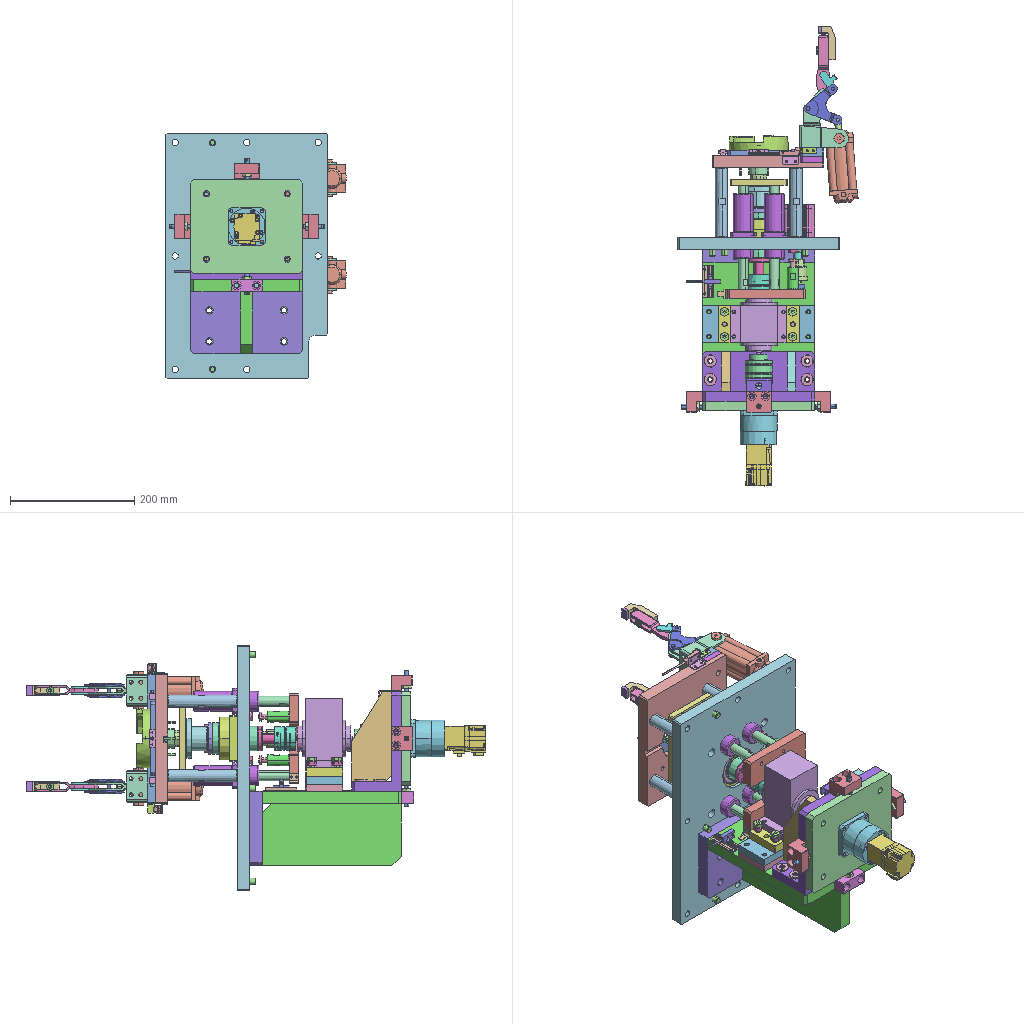Assembly | STEP file | 90 different items | 156 placed | box 290 x 740 x 395 mm
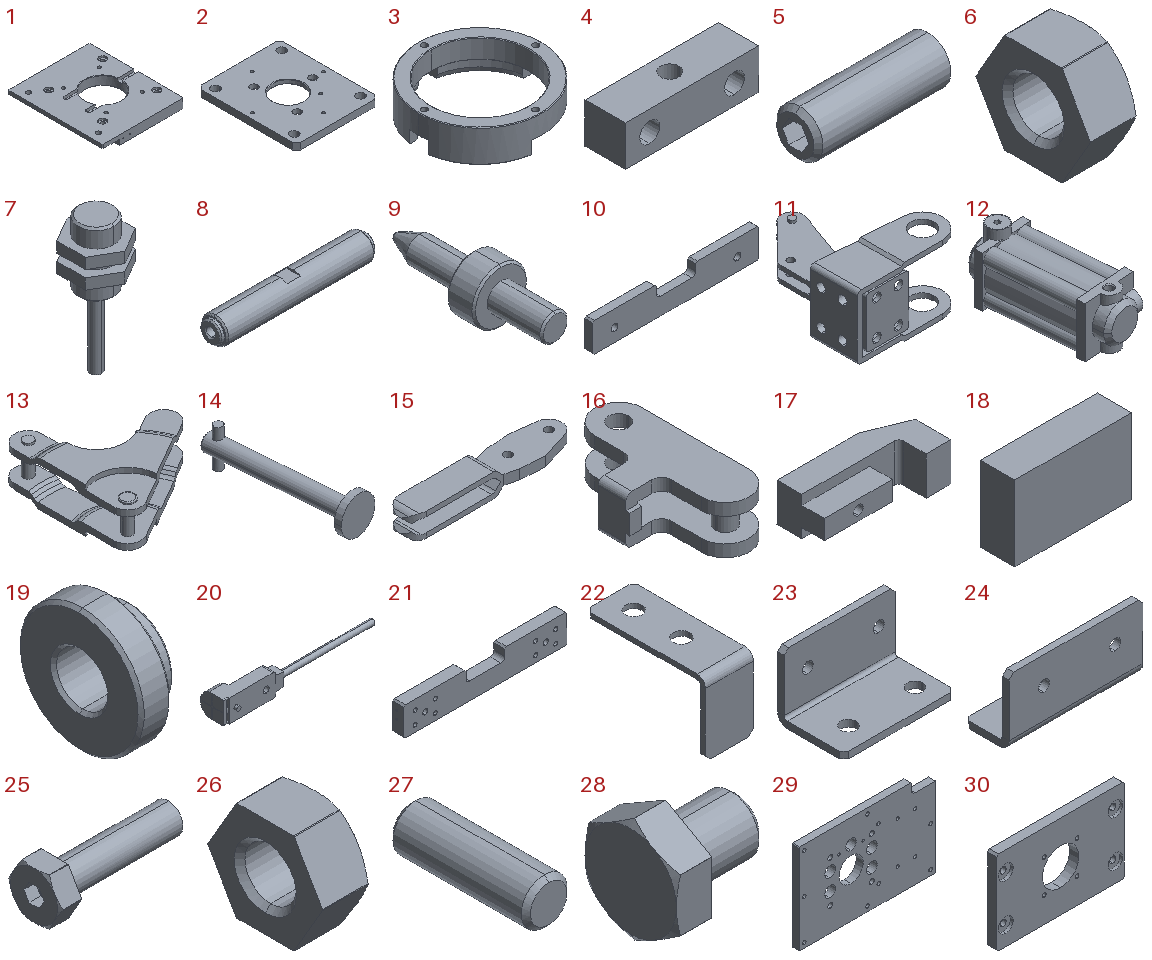Parts list (item | name | quantity | parent item | size | volume):
1 | PN_0012 Base | x1 | in PN_0040 JIG Assy | 180 x 210 x 20 mm | 540025 mm3
2 | PN_0030 JIG Plate | x1 | in PN_0040 JIG Assy | 100 x 120 x 8 mm | 64897 mm3
3 | PN_0005 JIG | x1 | in PN_0040 JIG Assy | 95 x 95 x 25 mm | 47843 mm3
4 | SceondTSE6-8_Default | x4 | in PN_0040 JIG Assy | 30 x 9 x 9 mm | 1675 mm3
5 | Sceond1_8 | x3 | in Sceondanbn5_15_2_03 | 15 x 5 x 5 mm | 269.138 mm3
6 | Sceond2_8 | x3 | in Sceondanbn5_15_2_03 | 4 x 9.2 x 8 mm | 164.255 mm3
7 | SceondEH-110 | x3 | in PN_0040 JIG Assy | 14 x 16.166 x 38 mm | 2114 mm3
8 | sfph20_112_f3_p16_m8_t3_sc50_2_03 | x4 | in PN_0040 JIG Assy | 118 x 20 x 20 mm | 34479 mm3
9 | PN_0028 Pin_Default | x1 | in PN_0040 JIG Assy | 6 x 17.694 x 6 mm | 173.525 mm3
10 | PN_0016 Cylinder Plate_Default | x1 | in EWTYY_Default | 210 x 10 x 37 mm | 69052 mm3
11 | Sceond_200_APVM -1 | x2 | in Sceond200_APVM0_2_03 | 78.4 x 96 x 51 mm | 41940 mm3
12 | Sceond_200_APVM0 -5 | x2 | in Sceond200_APVM0_2_03 | 53.168 x 117.344 x 59.5 mm | 144246 mm3
13 | Sceond_200_APVM0 -4 | x2 | in Sceond200_APVM0_2_03 | 58.167 x 65 x 23 mm | 11402 mm3
14 | Sceond_200_APVM0 -2 | x2 | in Sceond200_APVM0_2_03 | 22.523 x 84.663 x 23 mm | 8038 mm3
15 | Sceond_200_APVM-6 | x2 | in Sceond200_APVM0_2_03 | 102.5 x 23 x 14.5 mm | 10818 mm3
16 | Sceond_200_APVM0 -3 | x2 | in Sceond200_APVM0_2_03 | 21 x 38.8 x 12 mm | 3137 mm3
17 | PN_0002  Clamp_Default | x2 | in Sceond200_APVM0_2_03 | 54 x 23 x 17 mm | 13573 mm3
18 | PN_0019 Block_Default | x2 | in Sceond200_APVM0_2_03 | 17 x 5 x 11 mm | 935 mm3
19 | ftcm_d8_5_h12_v5_0_t3_0_l5_0_2_03 | x2 | in Sceond200_APVM0_2_03 | 5 x 12 x 12 mm | 348.627 mm3
20 | gx-h12a | x2 | in EWTYY_Default | 81.8 x 14.5 x 12 mm | 2908 mm3
21 | PN_0021 Cylinder Plate_Default | x1 | in EWTYY_Default | 210 x 14 x 37 mm | 94894 mm3
22 | PN_0006 BKT | x2 | in EWTYY_Default | 10 x 25 x 15 mm | 363.45 mm3
23 | PN_0029 BKT | x1 | in EWTYY_Default | 25 x 15 x 15 mm | 998.233 mm3
24 | PN_0035 BKT | x1 | in EWTYY_Default | 30 x 10 x 15 mm | 982.198 mm3
25 | 1_2 | x1 | in anhn5_20_2_03 | 23.5 x 9.2 x 8 mm | 562.948 mm3
26 | 2_2 | x1 | in anhn5_20_2_03 | 4 x 9.2 x 8 mm | 164.832 mm3
27 | PH10-30_Default | x4 | in PN_0040 JIG Assy | 10 x 30 x 10 mm | 2327 mm3
28 | stehn13_2_03 | x2 | in PN_0040 JIG Assy | 15 x 13 x 15 mm | 1216 mm3
29 | (+2 more in 1 file) PN_0041 Base_Default | x1 | in PN_0040 JIG Assy | 395 x 20 x 260 mm | 1820392 mm3
30 | PN_0037 Plate_Default | x1 | in PN_0023 Upraise Assy_Default | 140 x 10 x 92 mm | 111742 mm3
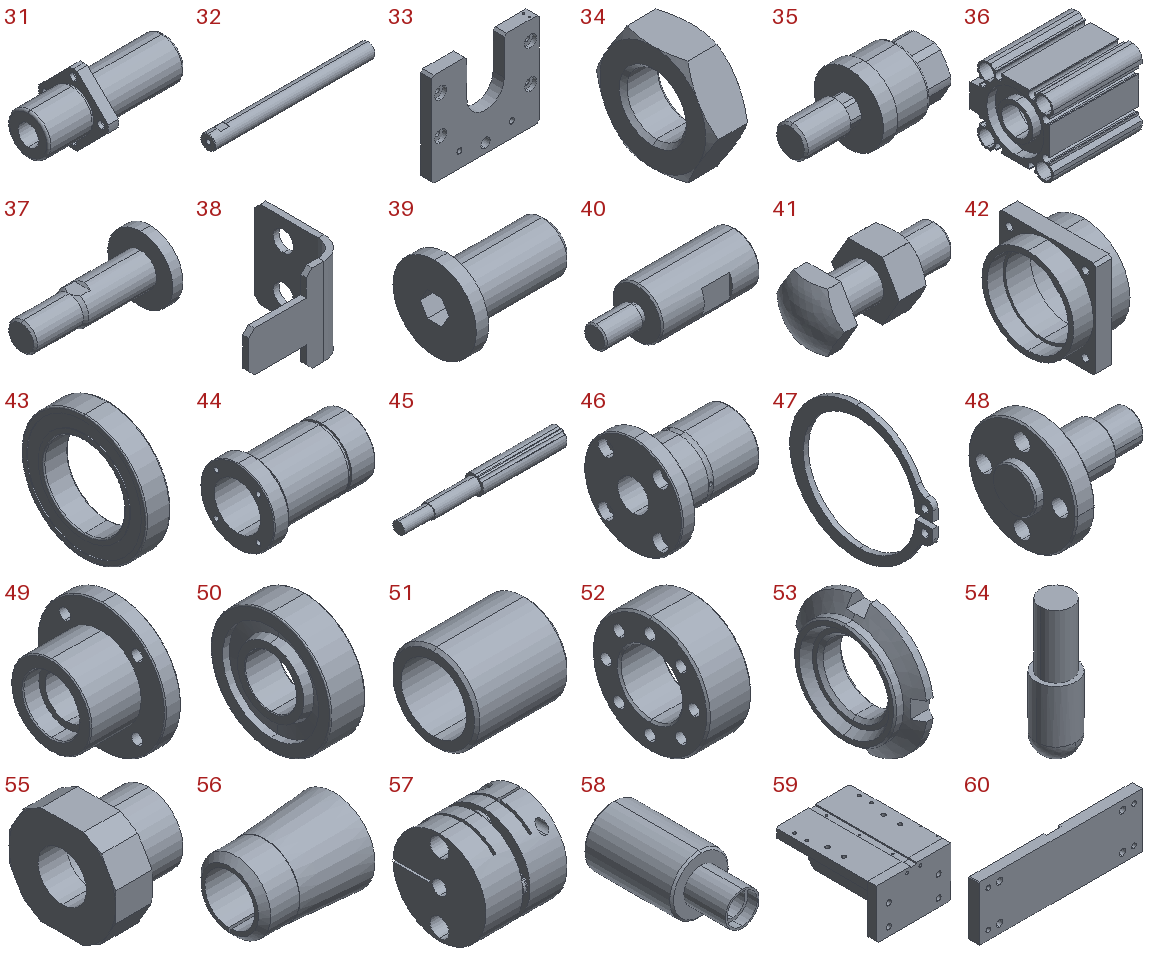31 | LHKMSNLF16 | x4 | in PN_0023 Upraise Assy_Default | 105 x 54 x 54 mm | 68941 mm3
32 | sfjz16_175_m6_n6_sc10_2_03 | x4 | in PN_0023 Upraise Assy_Default | 175 x 16 x 16 mm | 34378 mm3
33 | PN_0003 Plate_Default | x1 | in PN_0023 Upraise Assy_Default | 144 x 15 x 125 mm | 209014 mm3
34 | SceondHI_NT-04(CQ2)_Default | x1 | in PN_0023 Upraise Assy_Default | 8 x 25.403 x 22 mm | 2341 mm3
35 | - | x1 | in PN_0023 Upraise Assy_Default | 60 x 31 x 31 mm | 22129 mm3
36 | SceondHI_CDQ2B32-20CM-A93(0_0)_BODY_Default | x1 | - | 53 x 49.5 x 45 mm | 58938 mm3
37 | SceondHI_CDQ2B32-20CMA93(0_0)_CYROD_Default | x1 | - | 63.5 x 32 x 32 mm | 14555 mm3
38 | PN_0031 Sensor BKT_Default | x1 | in PN_0023 Upraise Assy_Default | 17 x 15 x 15 mm | 340.225 mm3
39 | cbss6_12_2_03 | x4 | in PN_0023 Upraise Assy_Default | 13.5 x 10 x 10 mm | 420.837 mm3
40 | PN_0032 Shaft_Default | x2 | in PN_0023 Upraise Assy_Default | 50 x 18 x 18 mm | 8746 mm3
41 | stbb8_25 | x2 | in PN_0023 Upraise Assy_Default | 30.458 x 15 x 13 mm | 2617 mm3
42 | PN_0025 Bearing Block_Default | x1 | in PN_0022 Rotary Assy_Default | 43 x 74 x 74 mm | 59989 mm3
43 | B6908ZZ_Default | x2 | in PN_0022 Rotary Assy_Default | 12 x 62 x 62 mm | 20172 mm3
44 | PN_0039 Shaft_Default | x1 | in PN_0022 Rotary Assy_Default | 73 x 50 x 50 mm | 53647 mm3
45 | SceondHI_LTR 16A150 LTRA Shaft_Default | x1 | - | 135 x 16 x 16 mm | 20071 mm3
46 | SceondHI_LF 16 FTLF Cylindar_Default | x1 | - | 50 x 51 x 51 mm | 35392 mm3
47 | SceondSTWN40_Default | x1 | in PN_0022 Rotary Assy_Default | 1.75 x 48.3 x 44.75 mm | 824.122 mm3
48 | PN_0036 Shaft_Default | x1 | in PN_0022 Rotary Assy_Default | 42 x 40 x 40 mm | 13938 mm3
49 | PN_0033 Bearing Block_Default | x1 | in PN_0022 Rotary Assy_Default | 33 x 64 x 64 mm | 39989 mm3
50 | b7001su | x2 | in PN_0022 Rotary Assy_Default | 8 x 28 x 28 mm | 3327 mm3
51 | CLBU12-16-3 | x1 | in PN_0022 Rotary Assy_Default | 17 x 16 x 16 mm | 1483 mm3
52 | PN_0034 JIG Block_Default | x1 | in PN_0022 Rotary Assy_Default | 12 x 32 x 32 mm | 6210 mm3
53 | funt12_2_03 | x1 | in PN_0022 Rotary Assy_Default | 5.4 x 21.794 x 21.794 mm | 953.545 mm3
54 | CKFQAGG3-P3.8-L6-B5_Default | x8 | in PN_0022 Rotary Assy_Default | 3.8 x 3.8 x 12.9 mm | 113.483 mm3
55 | 1_6 | x1 | in mlnp10_2_03 | 21 x 26 x 24 mm | 4121 mm3
56 | 2_6 | x1 | in mlnp10_2_03 | 21 x 16.3 x 16.296 mm | 1933 mm3
57 | SFC-035SA2-6B-12B_2_03 | x1 | in PN_0022 Rotary Assy_Default | 34 x 39 x 39 mm | 30442 mm3
58 | PN_0009 Center JIG_Default | x1 | in PN_0022 Rotary Assy_Default | 31 x 69 x 31 mm | 37981 mm3
59 | PN_0008 BKT_Default | x1 | in PN_0001 Drive Assy_Default | 180 x 244 x 120 mm | 1633565 mm3
60 | PN_0011 Plate 1_Default | x1 | in PN_0001 Drive Assy_Default | 180 x 11 x 60 mm | 113436 mm3
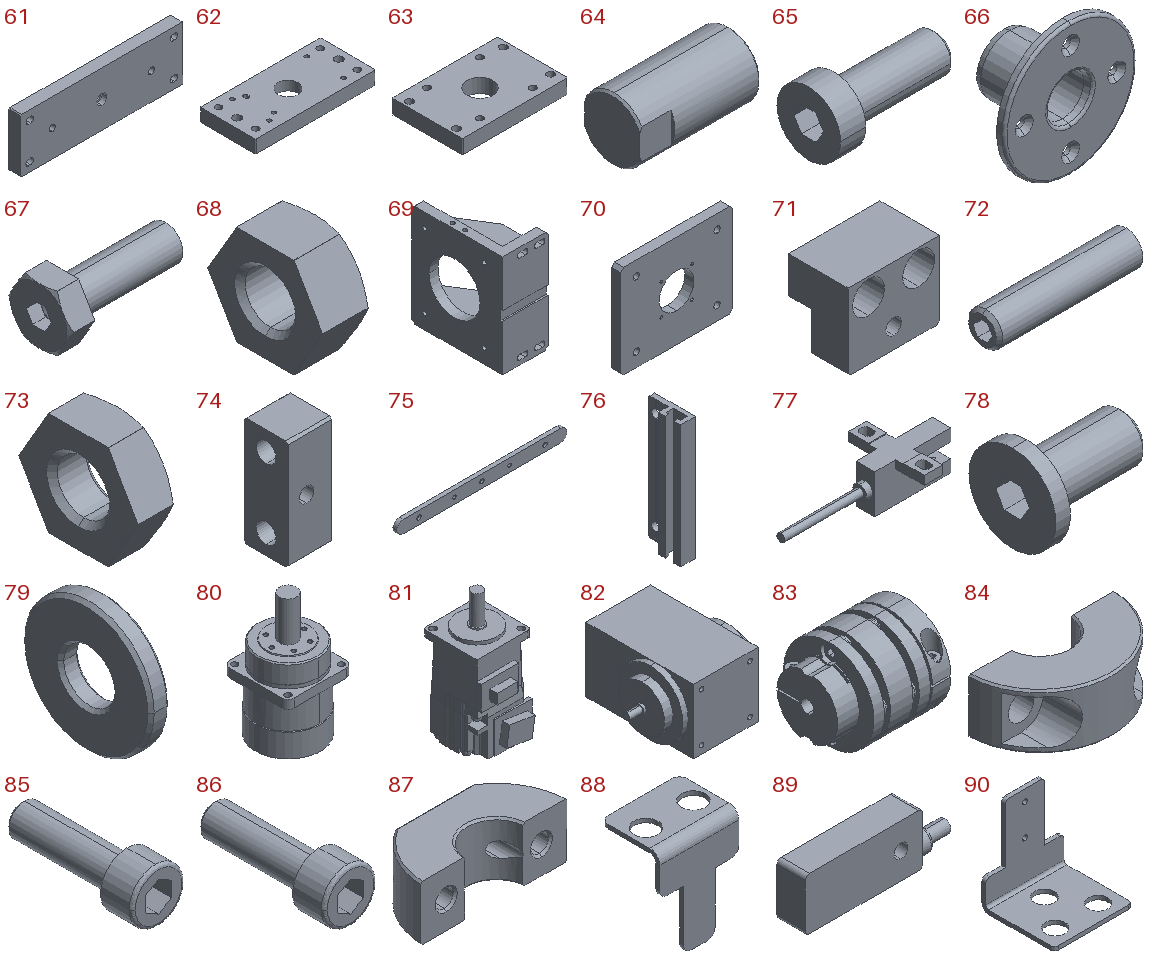61 | PN_0014 Plate 2_Default | x1 | in PN_0001 Drive Assy_Default | 180 x 13 x 60 mm | 135779 mm3
62 | PN_0013 Plate 3_Default | x1 | in PN_0001 Drive Assy_Default | 130 x 60 x 14 mm | 92668 mm3
63 | PN_0004 Plate 4_Default | x1 | in PN_0001 Drive Assy_Default | 90 x 60 x 12 mm | 56425 mm3
64 | PN_0024 Shaft_Default | x1 | in PN_0001 Drive Assy_Default | 30 x 16 x 16 mm | 5731 mm3
65 | CBSH6-16 | x1 | in PN_0001 Drive Assy_Default | 20 x 10 x 10 mm | 719.687 mm3
66 | MPSZ16-12_Default | x1 | in PN_0001 Drive Assy_Default | 50 x 25 x 50 mm | 8876 mm3
67 | Sceond1_7 | x4 | in Sceondanhn8_25_2_03 | 30.5 x 15 x 13 mm | 1960 mm3
68 | Sceond2_7 | x4 | in Sceondanhn8_25_2_03 | 6.5 x 15 x 13 mm | 713.15 mm3
69 | PN_0017 Motor BKT_Default | x1 | in PN_0001 Drive Assy_Default | 80 x 160 x 180 mm | 722805 mm3
70 | PN_0020 Motor Plate_Default | x1 | in PN_0001 Drive Assy_Default | 180 x 15 x 150 mm | 361761 mm3
71 | PN_0015 Block_Default | x3 | in PN_0001 Drive Assy_Default | 40 x 26 x 33.5 mm | 22128 mm3
72 | 1_11 | x4 | in anbnm8_35_2_03 | 35 x 8 x 8 mm | 1662 mm3
73 | 2_11 | x4 | in anbnm8_35_2_03 | 5 x 15 x 13 mm | 545.323 mm3
74 | PN_0010 Block_Default | x1 | in PN_0001 Drive Assy_Default | 20 x 20 x 50 mm | 14883 mm3
75 | PN_0027 KEY_Default | x1 | in PN_0001 Drive Assy_Default | 216 x 5 x 16 mm | 16228 mm3
76 | PN_0026 Sensor BKT | x1 | in Sensor Assy_Default | 6 x 17 x 50 mm | 2341 mm3
77 | PM-T44 | x1 | in Sensor Assy_Default | 55.2 x 26 x 13.7 mm | 2450 mm3
78 | cbss5_10_2_03 | x3 | in PN_0001 Drive Assy_Default | 11.5 x 9 x 9 mm | 264.715 mm3
79 | wssm20_8_3_2_03 | x4 | in PN_0001 Drive Assy_Default | 3 x 20 x 20 mm | 769.69 mm3
80 | PN_0007_Flange-Body201 | x1 | in PN_0007CSF-14-50-GH-F0ACD-100-HC-KFS_2_03 | 60 x 60 x 113 mm | 194551 mm3
81 | PN_0007hg-kr053_ | x1 | in PN_0001 Drive Assy_Default | 41.201 x 49.5 x 91.4 mm | 107634 mm3
82 | PN_0007TM301_Default | x1 | in PN_0001 Drive Assy_Default | 114 x 100 x 60 mm | 410522 mm3
83 | SFC-040DA2-6B-16B_2_03 | x1 | in PN_0001 Drive Assy_Default | 48 x 44 x 44 mm | 46226 mm3
84 | 1_3 | x1 | in sdn16_2_03_Default | 39.972 x 19.25 x 15 mm | 5522 mm3
85 | 2_3 | x1 | in sdn16_2_03_Default | 10 x 26 x 10 mm | 942.975 mm3
86 | 3_2 | x1 | in sdn16_2_03_Default | 10 x 26 x 10 mm | 942.975 mm3
87 | 4 | x1 | in sdn16_2_03_Default | 39.972 x 16.25 x 15 mm | 6108 mm3
88 | PN_0018 Sensor DOG_Default | x1 | in sdn16_2_03_Default | 20 x 15 x 25 mm | 521.133 mm3
89 | APS4-12S-Z_Default | x1 | - | 35 x 6.5 x 12 mm | 2071 mm3
90 | PN_0038 Sensor BKT_Default | x1 | - | 40 x 37 x 45 mm | 4613 mm3
Placements (level | parent | child | x y z in mm | rotation matrix by rows):
1 | subassembly 2 | PN_0040 JIG Assy | -0.0 148.0 85.0 | -1 0 0 0 0 -1 0 -1 0
2 | PN_0040 JIG Assy | PN_0012 Base | -0.0 -0.0 -0.0 | 1 0 0 0 1 0 0 0 1
2 | PN_0040 JIG Assy | PN_0030 JIG Plate | -0.0 -0.0 -8.0 | 1 0 0 0 1 0 0 0 1
2 | PN_0040 JIG Assy | PN_0005 JIG | 0.0 -0.0 -15.0 | 1 0 0 0 1 0 0 0 1
2 | PN_0040 JIG Assy | SceondTSE6-8_Default | -0.0 67.5 -4.0 | 1 0 0 0 0 1 0 -1 0
2 | PN_0040 JIG Assy | SceondTSE6-8_Default | -57.5 -0.0 -4.0 | 0 0 -1 1 0 0 0 -1 -0
2 | PN_0040 JIG Assy | SceondTSE6-8_Default | -0.0 -67.5 -4.0 | 1 0 0 0 0 1 0 -1 -0
2 | PN_0040 JIG Assy | SceondTSE6-8_Default | 57.5 -0.0 -4.0 | 0 0 1 -1 0 0 0 -1 -0
2 | PN_0040 JIG Assy | Sceondanbn5_15_2_03 | 65.0 -0.0 -9.0 | -1 0 0 0 0.5909 -0.8068 0 -0.8068 -0.5909
3 | Sceondanbn5_15_2_03 | Sceond1_8 | -0.0 -0.0 -0.0 | 1 0 0 0 1 0 0 0 1
3 | Sceondanbn5_15_2_03 | Sceond2_8 | -0.0 -0.0 -0.0 | 1 0 0 0 1 0 0 0 1
2 | PN_0040 JIG Assy | Sceondanbn5_15_2_03 | -0.0 77.5 -9.0 | 0 1 0 -1 0 0 0 0 1
3 | Sceondanbn5_15_2_03 | Sceond1_8 | -0.0 -0.0 -0.0 | 1 0 0 0 1 0 0 0 1
3 | Sceondanbn5_15_2_03 | Sceond2_8 | -0.0 -0.0 -0.0 | 1 0 0 0 1 0 0 0 1
2 | PN_0040 JIG Assy | Sceondanbn5_15_2_03 | -0.0 -77.5 -9.0 | 0 -0.6091 -0.7931 1 0 0 0 -0.7931 0.6091
3 | Sceondanbn5_15_2_03 | Sceond1_8 | -0.0 -0.0 -0.0 | 1 0 0 0 1 0 0 0 1
3 | Sceondanbn5_15_2_03 | Sceond2_8 | -0.0 -0.0 -0.0 | 1 0 0 0 1 0 0 0 1
2 | PN_0040 JIG Assy | SceondEH-110 | 30.0 0.0 -10.0 | 0.9796 -0.2008 0 -0.2008 -0.9796 0 0 0 -1
2 | PN_0040 JIG Assy | SceondEH-110 | -15.0 -25.981 -10.0 | 0.2954 0.9554 0 0.9554 -0.2954 0 0 0 -1
2 | PN_0040 JIG Assy | SceondEH-110 | -15.0 25.981 -10.0 | 0.9796 -0.2008 0 -0.2008 -0.9796 0 0 0 -1
2 | PN_0040 JIG Assy | sfph20_112_f3_p16_m8_t3_sc50_2_03 | -60.0 60.0 16.0 | 0 0.9897 0.1433 0 -0.1433 0.9897 1 0 0
2 | PN_0040 JIG Assy | sfph20_112_f3_p16_m8_t3_sc50_2_03 | 60.0 -60.0 16.0 | 0 0.9897 0.1433 0 -0.1433 0.9897 1 0 0
2 | PN_0040 JIG Assy | sfph20_112_f3_p16_m8_t3_sc50_2_03 | -60.0 -60.0 16.0 | 0 0.9897 0.1433 0 -0.1433 0.9897 1 0 0
2 | PN_0040 JIG Assy | sfph20_112_f3_p16_m8_t3_sc50_2_03 | 60.0 60.0 16.0 | 0 0.9897 0.1433 0 -0.1433 0.9897 1 0 0
2 | PN_0040 JIG Assy | PN_0028 Pin_Default | 17.998 -21.449 -6.0 | -0.3696 0 0.9292 -0.9292 0 -0.3696 0 -1 0
2 | PN_0040 JIG Assy | EWTYY_Default | -86.5 0.0 8.0 | 0 0 1 -1 0 0 0 -1 -0
3 | EWTYY_Default | PN_0016 Cylinder Plate_Default | -0.0 -0.0 -0.0 | 1 0 0 0 1 0 0 0 1
3 | EWTYY_Default | Sceond200_APVM0_2_03 | 77.103 24.0 19.603 | 0 0 1 0 1 0 -1 0 0
4 | Sceond200_APVM0_2_03 | Sceond_200_APVM -1 | 2.603 -0.0 0.3975 | 1 0 0 0 1 0 0 0 1
4 | Sceond200_APVM0_2_03 | Sceond_200_APVM0 -5 | 38.603 88.0 0.3975 | 1 0 0 0 1 0 0 0 1
4 | Sceond200_APVM0_2_03 | Sceond_200_APVM0 -4 | 48.382 58.532 0.3975 | 0.6272 0.7788 0 -0.7788 0.6272 0 0 0 1
4 | Sceond200_APVM0_2_03 | Sceond_200_APVM0 -2 | 42.077 44.159 0.3975 | 1 0 0 0 1 0 0 0 1
4 | Sceond200_APVM0_2_03 | Sceond_200_APVM-6 | 38.603 88.0 0.3975 | 0 1 0 -1 0 0 0 0 1
4 | Sceond200_APVM0_2_03 | Sceond_200_APVM0 -3 | 16.273 102.363 0.3975 | -0.8308 0.5566 0 -0.5566 -0.8308 0 0 0 1
4 | Sceond200_APVM0_2_03 | PN_0002  Clamp_Default | 56.603 142.022 0.3975 | 0 1 0 1 0 0 0 0 -1
4 | Sceond200_APVM0_2_03 | PN_0019 Block_Default | 33.603 190.522 0.3975 | 0 -1 0 0 0 1 -1 0 -0
4 | Sceond200_APVM0_2_03 | ftcm_d8_5_h12_v5_0_t3_0_l5_0_2_03 | 25.603 157.022 0.3975 | 1 0 0 0 1 0 0 0 1
3 | EWTYY_Default | Sceond200_APVM0_2_03 | -77.897 24.0 19.603 | 0 0 1 0 1 0 -1 0 0
4 | Sceond200_APVM0_2_03 | Sceond_200_APVM -1 | 2.603 -0.0 0.3975 | 1 0 0 0 1 0 0 0 1
4 | Sceond200_APVM0_2_03 | Sceond_200_APVM0 -5 | 38.603 88.0 0.3975 | 1 0 0 0 1 0 0 0 1
4 | Sceond200_APVM0_2_03 | Sceond_200_APVM0 -4 | 48.382 58.532 0.3975 | 0.6272 0.7788 0 -0.7788 0.6272 0 0 0 1
4 | Sceond200_APVM0_2_03 | Sceond_200_APVM0 -2 | 42.077 44.159 0.3975 | 1 0 0 0 1 0 0 0 1
4 | Sceond200_APVM0_2_03 | Sceond_200_APVM-6 | 38.603 88.0 0.3975 | 0 1 0 -1 0 0 0 0 1
4 | Sceond200_APVM0_2_03 | Sceond_200_APVM0 -3 | 16.273 102.363 0.3975 | -0.8308 0.5566 0 -0.5566 -0.8308 0 0 0 1
4 | Sceond200_APVM0_2_03 | PN_0002  Clamp_Default | 56.603 142.022 0.3975 | 0 1 0 1 0 0 0 0 -1
4 | Sceond200_APVM0_2_03 | PN_0019 Block_Default | 33.603 190.522 0.3975 | 0 -1 0 0 0 1 -1 0 -0
4 | Sceond200_APVM0_2_03 | ftcm_d8_5_h12_v5_0_t3_0_l5_0_2_03 | 25.603 157.022 0.3975 | 1 0 0 0 1 0 0 0 1
3 | EWTYY_Default | gx-h12a | 114.0 12.0 42.7 | 0 0 -1 0 1 0 1 0 0
3 | EWTYY_Default | gx-h12a | -114.0 2.0 42.7 | 0 0 -1 0 1 0 1 0 0
3 | EWTYY_Default | PN_0021 Cylinder Plate_Default | -0.0 10.0 -0.0 | 1 0 0 0 1 0 0 0 1
3 | EWTYY_Default | PN_0006 BKT | 105.0 14.0 18.5 | 0 0 -1 1 0 0 0 -1 0
3 | EWTYY_Default | PN_0029 BKT | 105.0 12.0 48.0 | 0 0 1 0 1 0 -1 0 0
3 | EWTYY_Default | PN_0035 BKT | -105.0 2.0 50.5 | 0 0 -1 0 -1 0 -1 0 0
3 | EWTYY_Default | PN_0006 BKT | -105.0 24.0 18.5 | 0 0 1 -1 0 0 0 -1 -0
2 | PN_0040 JIG Assy | anhn5_20_2_03 | -73.429 -0.0 -9.0 | 1 0 0 0 -0.4738 -0.8806 0 0.8806 -0.4738
3 | anhn5_20_2_03 | 1_2 | -0.0 -0.0 -0.0 | 1 0 0 0 1 0 0 0 1
3 | anhn5_20_2_03 | 2_2 | -0.0 -0.0 -0.0 | 1 0 0 0 1 0 0 0 1
2 | PN_0040 JIG Assy | PH10-30_Default | 55.0 -135.0 128.0 | 1 0 0 0 0 -1 0 1 -0
2 | PN_0040 JIG Assy | PH10-30_Default | 55.0 230.0 128.0 | 1 0 0 0 0 -1 0 1 -0
2 | PN_0040 JIG Assy | PH10-30_Default | 75.0 80.0 128.0 | 1 0 0 0 0 -1 0 1 -0
2 | PN_0040 JIG Assy | PH10-30_Default | -75.0 79.428 128.0 | 1 0 0 0 0 -1 0 1 -0
2 | PN_0040 JIG Assy | stehn13_2_03 | -55.0 -35.0 148.0 | 0 0 1 0 1 0 -1 0 0
2 | PN_0040 JIG Assy | stehn13_2_03 | -55.0 35.0 148.0 | 0 0 1 0 1 0 -1 0 0
2 | PN_0040 JIG Assy | (+2 more in 1 file) PN_0041 Base_Default | 80.0 0.0 148.0 | 0 0 -1 1 0 0 0 -1 -0
1 | subassembly 2 | PN_0023 Upraise Assy_Default | 63.0 20.0 85.0 | 0 0 -1 0 1 0 1 0 0
2 | PN_0023 Upraise Assy_Default | PN_0037 Plate_Default | -0.0 93.5 63.0 | 1 0 0 0 1 0 0 0 1
2 | PN_0023 Upraise Assy_Default | LHKMSNLF16 | -60.0 0.0 88.0 | 0 -0.7071 -0.7071 1 0 0 0 -0.7071 0.7071
2 | PN_0023 Upraise Assy_Default | LHKMSNLF16 | 60.0 0.0 88.0 | 0 -0.7071 -0.7071 1 0 0 0 -0.7071 0.7071
2 | PN_0023 Upraise Assy_Default | LHKMSNLF16 | 60.0 0.0 38.0 | 0 -0.7071 -0.7071 1 0 0 0 -0.7071 0.7071
2 | PN_0023 Upraise Assy_Default | LHKMSNLF16 | -60.0 -0.0 38.0 | 0 -0.7071 -0.7071 1 0 0 0 -0.7071 0.7071
2 | PN_0023 Upraise Assy_Default | sfjz16_175_m6_n6_sc10_2_03 | 60.0 -88.5 88.0 | 0 0.4692 0.8831 1 0 0 0 0.8831 -0.4692
2 | PN_0023 Upraise Assy_Default | sfjz16_175_m6_n6_sc10_2_03 | 60.0 -88.5 38.0 | 0 0.9879 -0.1551 1 0 0 0 -0.1551 -0.9879
2 | PN_0023 Upraise Assy_Default | sfjz16_175_m6_n6_sc10_2_03 | -60.0 -88.5 38.0 | 0 0.7374 0.6755 1 0 0 0 0.6755 -0.7374
2 | PN_0023 Upraise Assy_Default | sfjz16_175_m6_n6_sc10_2_03 | -60.0 86.5 88.0 | 0 -0.8293 -0.5589 -1 0 0 0 0.5589 -0.8293
2 | PN_0023 Upraise Assy_Default | PN_0003 Plate_Default | -0.0 -83.5 63.0 | -1 0 0 0 -1 0 0 0 1
2 | PN_0023 Upraise Assy_Default | SceondHI_NT-04(CQ2)_Default | 0.0 -79.5 -0.0 | 0 -1 0 1 0 0 0 0 1
2 | PN_0023 Upraise Assy_Default | subassembly 3 | -0.0 -35.5 -0.0 | 0 -0.5655 0.8248 1 0 0 0 0.8248 0.5655
2 | PN_0023 Upraise Assy_Default | subassembly 4 | -0.0 -0.0 -0.0 | 0 0 -1 1 0 0 0 -1 0
3 | subassembly 4 | SceondHI_CDQ2B32-20CM-A93(0_0)_BODY_Default | -0.0 -0.0 -0.0 | 1 0 0 0 1 0 0 0 1
3 | subassembly 4 | SceondHI_CDQ2B32-20CMA93(0_0)_CYROD_Default | -20.0 -0.0 -0.0 | 1 0 0 0 0.305 -0.9524 0 0.9524 0.305
2 | PN_0023 Upraise Assy_Default | PN_0031 Sensor BKT_Default | -71.0 -91.0 121.5 | 0 1 0 0 0 -1 -1 0 -0
2 | PN_0023 Upraise Assy_Default | cbss6_12_2_03 | 60.0 91.5 88.0 | 0 1 0 -1 0 0 0 0 1
2 | PN_0023 Upraise Assy_Default | cbss6_12_2_03 | -60.0 91.5 88.0 | 0 1 0 -1 0 0 0 0 1
2 | PN_0023 Upraise Assy_Default | cbss6_12_2_03 | 60.0 91.5 38.0 | 0 1 0 -1 0 0 0 0 1
2 | PN_0023 Upraise Assy_Default | cbss6_12_2_03 | -60.0 91.5 38.0 | 0 1 0 -1 0 0 0 0 1
2 | PN_0023 Upraise Assy_Default | PN_0032 Shaft_Default | 35.0 -83.5 8.0 | 0 -1 0 1 0 0 0 0 1
2 | PN_0023 Upraise Assy_Default | PN_0032 Shaft_Default | -35.0 -83.5 8.0 | 0 -1 0 1 0 0 0 0 1
2 | PN_0023 Upraise Assy_Default | stbb8_25 | 35.0 -39.25 8.0 | 0 0.9697 0.2444 -1 0 0 0 -0.2444 0.9697
2 | PN_0023 Upraise Assy_Default | stbb8_25 | -35.0 -39.25 8.0 | 0 0.9697 0.2444 -1 0 0 0 -0.2444 0.9697
1 | subassembly 2 | PN_0022 Rotary Assy_Default | -0.0 20.0 85.0 | 1 0 0 0 -1 0 0 0 -1
2 | PN_0022 Rotary Assy_Default | PN_0025 Bearing Block_Default | -0.0 -0.0 -0.0 | 0 0 1 -1 0 0 0 -1 0
2 | PN_0022 Rotary Assy_Default | B6908ZZ_Default | -0.0 3.0 -0.0 | 0 -1 0 1 0 0 0 0 1
2 | PN_0022 Rotary Assy_Default | B6908ZZ_Default | 0.0 -28.0 -0.0 | 0 -1 0 1 0 0 0 0 1
2 | PN_0022 Rotary Assy_Default | PN_0039 Shaft_Default | 0.0 -40.0 -0.0 | 0 1 0 1 0 0 0 0 -1
2 | PN_0022 Rotary Assy_Default | subassembly 5 | -0.0 -110.343 0.0 | 0 0.1396 -0.9902 1 0 0 0 -0.9902 -0.1396
3 | subassembly 5 | SceondHI_LTR 16A150 LTRA Shaft_Default | -2.169 -0.0 -0.0 | 1 0 0 0 0.6695 -0.7429 0 0.7429 0.6695
3 | subassembly 5 | SceondHI_LF 16 FTLF Cylindar_Default | 63.343 -0.0 -0.0 | 1 0 0 0 0.9902 -0.1396 0 0.1396 0.9902
2 | PN_0022 Rotary Assy_Default | SceondSTWN40_Default | -0.0 15.725 -0.0 | 0 0.1669 0.986 -1 0 0 0 -0.986 0.1669
2 | PN_0022 Rotary Assy_Default | PN_0036 Shaft_Default | -0.0 33.0 -0.0 | 0 -0.7071 -0.7071 1 0 0 0 -0.7071 0.7071
2 | PN_0022 Rotary Assy_Default | PN_0033 Bearing Block_Default | 0.0 -81.511 0.0 | 0 -0.98 -0.1988 -1 0 0 0 0.1988 -0.98
2 | PN_0022 Rotary Assy_Default | b7001su | 0.0 -56.511 0.0 | 0 -1 0 1 0 0 0 0 1
2 | PN_0022 Rotary Assy_Default | b7001su | 0.0 -81.511 0.0 | 0 -1 0 1 0 0 0 0 1
2 | PN_0022 Rotary Assy_Default | CLBU12-16-3 | 0.0 -73.511 0.0 | 0 -1 0 1 0 0 0 0 1
2 | PN_0022 Rotary Assy_Default | PN_0034 JIG Block_Default | 0.0 -112.511 -0.0 | 0 0.934 -0.3573 1 0 0 0 -0.3573 -0.934
2 | PN_0022 Rotary Assy_Default | funt12_2_03 | 0.0 -81.511 0.0 | 0 0.8326 0.5539 -1 0 0 0 -0.5539 0.8326
2 | PN_0022 Rotary Assy_Default | CKFQAGG3-P3.8-L6-B5_Default | 4.287 -119.412 11.208 | -0.1711 -0.9852 0 0 0 1 -0.9852 0.1711 0
2 | PN_0022 Rotary Assy_Default | CKFQAGG3-P3.8-L6-B5_Default | -4.894 -119.412 10.957 | 0.5757 -0.8177 0 0 0 1 -0.8177 -0.5757 0
2 | PN_0022 Rotary Assy_Default | CKFQAGG3-P3.8-L6-B5_Default | -11.208 -119.412 4.287 | 0.9852 -0.1711 0 0 0 1 -0.1711 -0.9852 -0
2 | PN_0022 Rotary Assy_Default | CKFQAGG3-P3.8-L6-B5_Default | -10.957 -119.412 -4.894 | 0.8177 0.5757 0 0 0 1 0.5757 -0.8177 -0
2 | PN_0022 Rotary Assy_Default | CKFQAGG3-P3.8-L6-B5_Default | -4.287 -119.412 -11.208 | 0.1711 0.9852 0 0 0 1 0.9852 -0.1711 0
2 | PN_0022 Rotary Assy_Default | CKFQAGG3-P3.8-L6-B5_Default | 4.894 -119.412 -10.957 | -0.5757 0.8177 0 0 0 1 0.8177 0.5757 0
2 | PN_0022 Rotary Assy_Default | CKFQAGG3-P3.8-L6-B5_Default | 11.208 -119.412 -4.287 | -0.9852 0.1711 0 0 0 1 0.1711 0.9852 0
2 | PN_0022 Rotary Assy_Default | CKFQAGG3-P3.8-L6-B5_Default | 10.957 -119.412 4.894 | -0.8177 -0.5757 0 0 0 1 -0.5757 0.8177 0
2 | PN_0022 Rotary Assy_Default | mlnp10_2_03 | -0.0 -91.511 -0.0 | 0 -0.5086 0.861 -1 0 0 0 -0.861 -0.5086
3 | mlnp10_2_03 | 1_6 | -0.0 -0.0 -0.0 | 1 0 0 0 1 0 0 0 1
3 | mlnp10_2_03 | 2_6 | -0.0 -0.0 -0.0 | 1 0 0 0 1 0 0 0 1
2 | PN_0022 Rotary Assy_Default | SFC-035SA2-6B-12B_2_03 | -0.0 94.0 -0.0 | 0 0.3629 -0.9318 -1 0 0 0 0.9318 0.3629
2 | PN_0022 Rotary Assy_Default | PN_0009 Center JIG_Default | -0.0 33.0 0.0 | 0.6865 0 0.7271 0 -1 0 0.7271 0 -0.6865
1 | subassembly 2 | PN_0001 Drive Assy_Default | -0.0 -0.0 -0.0 | -1 0 0 0 -1 0 0 0 1
2 | PN_0001 Drive Assy_Default | PN_0008 BKT_Default | -0.0 -0.0 -0.0 | 1 0 0 0 1 0 0 0 1
2 | PN_0001 Drive Assy_Default | PN_0011 Plate 1_Default | -0.0 120.0 11.0 | 1 0 0 0 0 1 0 -1 0
2 | PN_0001 Drive Assy_Default | PN_0014 Plate 2_Default | -0.0 120.0 11.0 | 1 0 0 0 0 -1 0 1 -0
2 | PN_0001 Drive Assy_Default | PN_0013 Plate 3_Default | -0.0 120.0 24.0 | 1 0 0 0 1 0 0 0 1
2 | PN_0001 Drive Assy_Default | PN_0004 Plate 4_Default | -0.0 120.0 38.0 | 1 0 0 0 1 0 0 0 1
2 | PN_0001 Drive Assy_Default | PN_0024 Shaft_Default | -0.0 120.0 51.0 | 0 -0.9768 -0.2143 0 -0.2143 0.9768 -1 0 -0
2 | PN_0001 Drive Assy_Default | CBSH6-16 | -0.0 120.0 16.0 | 0 -0.4901 -0.8717 0 0.8717 -0.4901 1 0 -0
2 | PN_0001 Drive Assy_Default | MPSZ16-12_Default | -0.0 120.0 28.312 | 0.3925 0 0.9197 0.9197 0 -0.3925 0 1 -0
2 | PN_0001 Drive Assy_Default | Sceondanhn8_25_2_03 | 55.0 100.0 54.5 | 0 0.02553 0.9997 0 0.9997 -0.02553 -1 0 0
3 | Sceondanhn8_25_2_03 | Sceond1_7 | -0.0 -0.0 0.0 | 1 0 0 0 1 0 0 0 1
3 | Sceondanhn8_25_2_03 | Sceond2_7 | -7.679 -0.0 0.0 | 1 0 0 0 1 0 0 0 1
2 | PN_0001 Drive Assy_Default | Sceondanhn8_25_2_03 | -55.0 140.0 54.5 | 0 0.02553 0.9997 0 0.9997 -0.02553 -1 0 0
3 | Sceondanhn8_25_2_03 | Sceond1_7 | -0.0 -0.0 0.0 | 1 0 0 0 1 0 0 0 1
3 | Sceondanhn8_25_2_03 | Sceond2_7 | -7.679 -0.0 0.0 | 1 0 0 0 1 0 0 0 1
2 | PN_0001 Drive Assy_Default | Sceondanhn8_25_2_03 | -55.0 100.0 54.5 | 0 0.02553 0.9997 0 0.9997 -0.02553 -1 0 0
3 | Sceondanhn8_25_2_03 | Sceond1_7 | -0.0 -0.0 0.0 | 1 0 0 0 1 0 0 0 1
3 | Sceondanhn8_25_2_03 | Sceond2_7 | -7.679 -0.0 0.0 | 1 0 0 0 1 0 0 0 1
2 | PN_0001 Drive Assy_Default | Sceondanhn8_25_2_03 | 55.0 140.0 54.5 | 0 0.02553 0.9997 0 0.9997 -0.02553 -1 0 0
3 | Sceondanhn8_25_2_03 | Sceond1_7 | -0.0 -0.0 0.0 | 1 0 0 0 1 0 0 0 1
3 | Sceondanhn8_25_2_03 | Sceond2_7 | -7.679 -0.0 0.0 | 1 0 0 0 1 0 0 0 1
2 | PN_0001 Drive Assy_Default | PN_0017 Motor BKT_Default | -0.0 244.0 0.0 | 0 0 -1 -1 0 0 0 1 -0
2 | PN_0001 Drive Assy_Default | PN_0020 Motor Plate_Default | -0.0 259.0 85.0 | -1 0 0 0 -1 0 0 0 1
2 | PN_0001 Drive Assy_Default | PN_0015 Block_Default | -116.0 228.0 85.0 | 0 1 0 0 0 -1 -1 0 0
2 | PN_0001 Drive Assy_Default | PN_0015 Block_Default | 116.0 228.0 85.0 | 0 -1 0 0 0 -1 1 0 -0
2 | PN_0001 Drive Assy_Default | PN_0015 Block_Default | -0.0 228.0 186.0 | -1 0 0 0 0 -1 0 -1 0
2 | PN_0001 Drive Assy_Default | anbnm8_35_2_03 | 125.0 252.5 85.0 | -1 0 0 0 0.9758 0.2186 0 0.2186 -0.9758
3 | anbnm8_35_2_03 | 1_11 | -0.0 0.0 -0.0 | 1 0 0 0 1 0 0 0 1
3 | anbnm8_35_2_03 | 2_11 | 10.0 0.0 -0.0 | 1 0 0 0 1 0 0 0 1
2 | PN_0001 Drive Assy_Default | anbnm8_35_2_03 | -125.0 252.5 85.0 | 1 0 0 0 1 0 0 0 1
3 | anbnm8_35_2_03 | 1_11 | -0.0 0.0 -0.0 | 1 0 0 0 1 0 0 0 1
3 | anbnm8_35_2_03 | 2_11 | 10.0 0.0 -0.0 | 1 0 0 0 1 0 0 0 1
2 | PN_0001 Drive Assy_Default | anbnm8_35_2_03 | -0.0 252.5 195.0 | 0 0.766 -0.6428 0 -0.6428 -0.766 -1 0 0
3 | anbnm8_35_2_03 | 1_11 | -0.0 0.0 -0.0 | 1 0 0 0 1 0 0 0 1
3 | anbnm8_35_2_03 | 2_11 | 10.0 0.0 -0.0 | 1 0 0 0 1 0 0 0 1
2 | PN_0001 Drive Assy_Default | PN_0010 Block_Default | -0.0 244.0 -10.0 | 0 0 1 1 0 0 0 1 0
2 | PN_0001 Drive Assy_Default | anbnm8_35_2_03 | -0.0 252.5 -25.0 | 0 0.5746 0.8184 0 -0.8184 0.5746 1 0 0
3 | anbnm8_35_2_03 | 1_11 | -0.0 0.0 -0.0 | 1 0 0 0 1 0 0 0 1
3 | anbnm8_35_2_03 | 2_11 | 10.0 0.0 -0.0 | 1 0 0 0 1 0 0 0 1
2 | PN_0001 Drive Assy_Default | PN_0027 KEY_Default | 0.0 130.0 -3.0 | 0 0 -1 -1 0 0 0 1 -0
2 | PN_0001 Drive Assy_Default | Sensor Assy_Default | 90.0 76.0 -0.0 | 1 0 0 0 0 -1 0 1 0
3 | Sensor Assy_Default | PN_0026 Sensor BKT | 0.0 0.0 -0.0 | 0 1 0 -1 0 0 0 0 1
3 | Sensor Assy_Default | PM-T44 | -25.5 13.0 25.0 | -1 0 0 0 0 -1 0 -1 -0
2 | PN_0001 Drive Assy_Default | cbss5_10_2_03 | -0.0 50.0 0.0 | 0 0 1 0 1 0 -1 0 -0
2 | PN_0001 Drive Assy_Default | cbss5_10_2_03 | -0.0 130.0 -0.0 | 0 0 1 0 1 0 -1 0 -0
2 | PN_0001 Drive Assy_Default | cbss5_10_2_03 | 0.0 210.0 -0.0 | 0 0 1 0 1 0 -1 0 -0
2 | PN_0001 Drive Assy_Default | wssm20_8_3_2_03 | -78.0 179.0 16.0 | 0 0.03176 -0.9995 0 0.9995 0.03176 1 0 0
2 | PN_0001 Drive Assy_Default | wssm20_8_3_2_03 | 78.0 179.0 16.0 | 0 0.03176 -0.9995 0 0.9995 0.03176 1 0 0
2 | PN_0001 Drive Assy_Default | wssm20_8_3_2_03 | -78.0 209.0 16.0 | 0 0.03176 -0.9995 0 0.9995 0.03176 1 0 0
2 | PN_0001 Drive Assy_Default | wssm20_8_3_2_03 | 78.0 209.0 16.0 | 0 0.03176 -0.9995 0 0.9995 0.03176 1 0 0
2 | PN_0001 Drive Assy_Default | PN_0007CSF-14-50-GH-F0ACD-100-HC-KFS_2_03 | -0.0 238.0 85.0 | 0 -1 0 1 0 0 0 0 1
3 | PN_0007CSF-14-50-GH-F0ACD-100-HC-KFS_2_03 | PN_0007_Flange-Body201 | -0.0 -0.0 -0.0 | 0 0 -1 0 1 0 1 0 -0
2 | PN_0001 Drive Assy_Default | PN_0007hg-kr053_ | 0.0 314.0 85.0 | 1 0 0 0 0 -1 0 1 0
2 | PN_0001 Drive Assy_Default | PN_0007TM301_Default | 0.0 120.0 50.0 | 0 0 1 1 0 0 0 1 -0
2 | PN_0001 Drive Assy_Default | SFC-040DA2-6B-16B_2_03 | 0.0 168.0 85.0 | 0 0.08262 -0.9966 1 0 0 0 -0.9966 -0.08262
1 | subassembly 2 | sdn16_2_03_Default | 0.0 -225.5 85.0 | 1 0 0 0 0 -1 0 1 -0
2 | sdn16_2_03_Default | 1_3 | -0.0 -0.0 -0.0 | 1 0 0 0 1 0 0 0 1
2 | sdn16_2_03_Default | 2_3 | -0.0 -0.0 -0.0 | 1 0 0 0 1 0 0 0 1
2 | sdn16_2_03_Default | 3_2 | -0.0 -0.0 -0.0 | 1 0 0 0 1 0 0 0 1
2 | sdn16_2_03_Default | 4 | -0.0 -0.0 -0.0 | 1 0 0 0 1 0 0 0 1
2 | sdn16_2_03_Default | PN_0018 Sensor DOG_Default | -10.0 17.0 -7.5 | 1 0 0 0 0 -1 0 1 0
1 | subassembly 2 | APS4-12S-Z_Default | 0.0 -209.5 139.0 | 0 0 1 0 -1 0 1 0 -0
1 | subassembly 2 | PN_0038 Sensor BKT_Default | 20.0 -244.5 160.233 | -1 0 0 0 1 0 0 0 -1